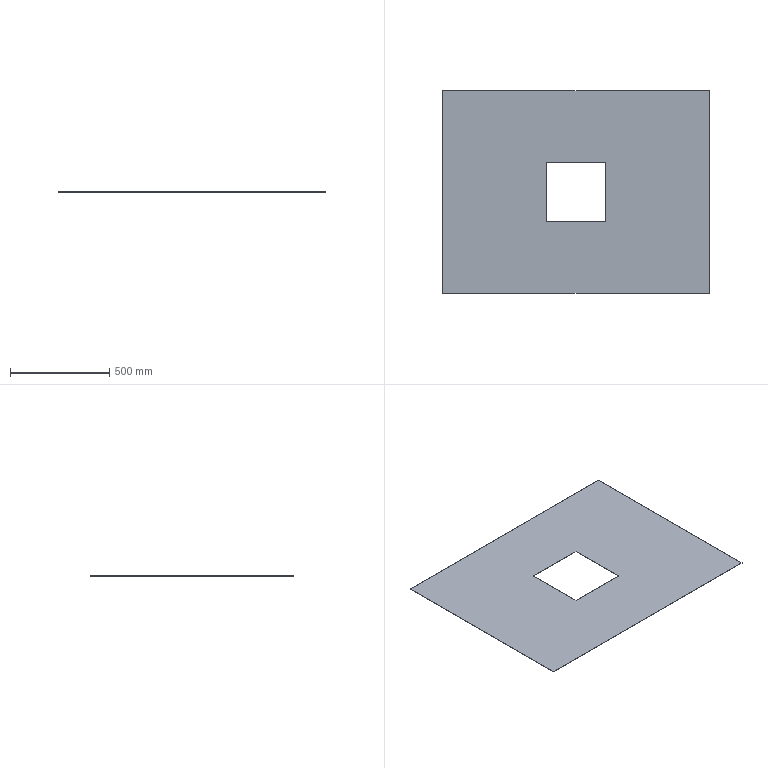Part | SolidWorks | features FlatPattern 1, SMBaseFlange 1, SheetMetal 1 | 1 solid | 10 faces | box 1345 x 1022 x 1.5 mm | volume 1927692 mm3 | plane 10
STEP:
#1=CARTESIAN_POINT('',(-672.5,0.,1.5));
#2=VERTEX_POINT('',#1);
#3=CARTESIAN_POINT('',(-672.5,-1022.4,1.5));
#4=VERTEX_POINT('',#3);
#5=CARTESIAN_POINT('',(-672.5,0.,1.5));
#6=DIRECTION('',(0.,-1.,0.));
#7=VECTOR('',#6,1000.);
#8=LINE('',#5,#7);
#9=EDGE_CURVE('',#2,#4,#8,.T.);
#10=ORIENTED_EDGE('',*,*,#9,.T.);
#11=CARTESIAN_POINT('',(672.5,-1022.4,1.5));
#12=VERTEX_POINT('',#11);
#13=CARTESIAN_POINT('',(-672.5,-1022.4,1.5));
#14=DIRECTION('',(1.,0.,0.));
#15=VECTOR('',#14,1000.);
#16=LINE('',#13,#15);
#17=EDGE_CURVE('',#4,#12,#16,.T.);
#18=ORIENTED_EDGE('',*,*,#17,.T.);
#19=CARTESIAN_POINT('',(672.5,0.,1.5));
#20=VERTEX_POINT('',#19);
#21=CARTESIAN_POINT('',(672.5,0.,1.5));
#22=DIRECTION('',(0.,1.,0.));
#23=VECTOR('',#22,1000.);
#24=LINE('',#21,#23);
#25=EDGE_CURVE('',#12,#20,#24,.T.);
#26=ORIENTED_EDGE('',*,*,#25,.T.);
#27=CARTESIAN_POINT('',(-672.5,0.,1.5));
#28=DIRECTION('',(-1.,0.,0.));
#29=VECTOR('',#28,1000.);
#30=LINE('',#27,#29);
#31=EDGE_CURVE('',#20,#2,#30,.T.);
#32=ORIENTED_EDGE('',*,*,#31,.T.);
#33=EDGE_LOOP('',(#10,#18,#26,#32));
#34=FACE_OUTER_BOUND('',#33,.T.);
#35=CARTESIAN_POINT('',(150.,-361.2,1.5));
#36=VERTEX_POINT('',#35);
#37=CARTESIAN_POINT('',(-150.,-361.2,1.5));
#38=VERTEX_POINT('',#37);
#39=CARTESIAN_POINT('',(-150.,-361.2,1.5));
#40=DIRECTION('',(-1.,0.,0.));
#41=VECTOR('',#40,1000.);
#42=LINE('',#39,#41);
#43=EDGE_CURVE('',#36,#38,#42,.T.);
#44=ORIENTED_EDGE('',*,*,#43,.F.);
#45=CARTESIAN_POINT('',(150.,-661.2,1.5));
#46=VERTEX_POINT('',#45);
#47=CARTESIAN_POINT('',(150.,-661.2,1.5));
#48=DIRECTION('',(0.,1.,0.));
#49=VECTOR('',#48,1000.);
#50=LINE('',#47,#49);
#51=EDGE_CURVE('',#46,#36,#50,.T.);
#52=ORIENTED_EDGE('',*,*,#51,.F.);
#53=CARTESIAN_POINT('',(-150.,-661.2,1.5));
#54=VERTEX_POINT('',#53);
#55=CARTESIAN_POINT('',(-150.,-661.2,1.5));
#56=DIRECTION('',(1.,0.,0.));
#57=VECTOR('',#56,1000.);
#58=LINE('',#55,#57);
#59=EDGE_CURVE('',#54,#46,#58,.T.);
#60=ORIENTED_EDGE('',*,*,#59,.F.);
#61=CARTESIAN_POINT('',(-150.,-661.2,1.5));
#62=DIRECTION('',(0.,-1.,0.));
#63=VECTOR('',#62,1000.);
#64=LINE('',#61,#63);
#65=EDGE_CURVE('',#38,#54,#64,.T.);
#66=ORIENTED_EDGE('',*,*,#65,.F.);
#67=EDGE_LOOP('',(#44,#52,#60,#66));
#68=FACE_BOUND('',#67,.T.);
#69=CARTESIAN_POINT('',(0.,0.,1.5));
#70=DIRECTION('',(0.,0.,1.));
#71=DIRECTION('',(1.,0.,0.));
#72=AXIS2_PLACEMENT_3D('',#69,#70,#71);
#73=PLANE('',#72);
#74=ADVANCED_FACE('',(#34,#68),#73,.T.);
#75=CARTESIAN_POINT('',(-672.5,0.,0.));
#76=VERTEX_POINT('',#75);
#77=CARTESIAN_POINT('',(-672.5,-1022.4,0.));
#78=VERTEX_POINT('',#77);
#79=CARTESIAN_POINT('',(-672.5,0.,0.));
#80=DIRECTION('',(0.,-1.,0.));
#81=VECTOR('',#80,1000.);
#82=LINE('',#79,#81);
#83=EDGE_CURVE('',#76,#78,#82,.T.);
#84=ORIENTED_EDGE('',*,*,#83,.F.);
#85=CARTESIAN_POINT('',(672.5,0.,0.));
#86=VERTEX_POINT('',#85);
#87=CARTESIAN_POINT('',(-672.5,0.,0.));
#88=DIRECTION('',(-1.,0.,0.));
#89=VECTOR('',#88,1000.);
#90=LINE('',#87,#89);
#91=EDGE_CURVE('',#86,#76,#90,.T.);
#92=ORIENTED_EDGE('',*,*,#91,.F.);
#93=CARTESIAN_POINT('',(672.5,-1022.4,0.));
#94=VERTEX_POINT('',#93);
#95=CARTESIAN_POINT('',(672.5,0.,0.));
#96=DIRECTION('',(0.,1.,0.));
#97=VECTOR('',#96,1000.);
#98=LINE('',#95,#97);
#99=EDGE_CURVE('',#94,#86,#98,.T.);
#100=ORIENTED_EDGE('',*,*,#99,.F.);
#101=CARTESIAN_POINT('',(-672.5,-1022.4,0.));
#102=DIRECTION('',(1.,0.,0.));
#103=VECTOR('',#102,1000.);
#104=LINE('',#101,#103);
#105=EDGE_CURVE('',#78,#94,#104,.T.);
#106=ORIENTED_EDGE('',*,*,#105,.F.);
#107=EDGE_LOOP('',(#84,#92,#100,#106));
#108=FACE_OUTER_BOUND('',#107,.T.);
#109=CARTESIAN_POINT('',(150.,-661.2,0.));
#110=VERTEX_POINT('',#109);
#111=CARTESIAN_POINT('',(150.,-361.2,0.));
#112=VERTEX_POINT('',#111);
#113=CARTESIAN_POINT('',(150.,-661.2,0.));
#114=DIRECTION('',(0.,1.,0.));
#115=VECTOR('',#114,1000.);
#116=LINE('',#113,#115);
#117=EDGE_CURVE('',#110,#112,#116,.T.);
#118=ORIENTED_EDGE('',*,*,#117,.T.);
#119=CARTESIAN_POINT('',(-150.,-361.2,0.));
#120=VERTEX_POINT('',#119);
#121=CARTESIAN_POINT('',(-150.,-361.2,0.));
#122=DIRECTION('',(-1.,0.,0.));
#123=VECTOR('',#122,1000.);
#124=LINE('',#121,#123);
#125=EDGE_CURVE('',#112,#120,#124,.T.);
#126=ORIENTED_EDGE('',*,*,#125,.T.);
#127=CARTESIAN_POINT('',(-150.,-661.2,0.));
#128=VERTEX_POINT('',#127);
#129=CARTESIAN_POINT('',(-150.,-661.2,0.));
#130=DIRECTION('',(0.,-1.,0.));
#131=VECTOR('',#130,1000.);
#132=LINE('',#129,#131);
#133=EDGE_CURVE('',#120,#128,#132,.T.);
#134=ORIENTED_EDGE('',*,*,#133,.T.);
#135=CARTESIAN_POINT('',(-150.,-661.2,0.));
#136=DIRECTION('',(1.,0.,0.));
#137=VECTOR('',#136,1000.);
#138=LINE('',#135,#137);
#139=EDGE_CURVE('',#128,#110,#138,.T.);
#140=ORIENTED_EDGE('',*,*,#139,.T.);
#141=EDGE_LOOP('',(#118,#126,#134,#140));
#142=FACE_BOUND('',#141,.T.);
#143=CARTESIAN_POINT('',(0.,0.,0.));
#144=DIRECTION('',(0.,0.,1.));
#145=DIRECTION('',(1.,0.,0.));
#146=AXIS2_PLACEMENT_3D('',#143,#144,#145);
#147=PLANE('',#146);
#148=ADVANCED_FACE('',(#108,#142),#147,.F.);
#149=ORIENTED_EDGE('',*,*,#83,.T.);
#150=CARTESIAN_POINT('',(-672.5,-1022.4,1.5));
#151=DIRECTION('',(0.,0.,-1.));
#152=VECTOR('',#151,1000.);
#153=LINE('',#150,#152);
#154=EDGE_CURVE('',#4,#78,#153,.T.);
#155=ORIENTED_EDGE('',*,*,#154,.F.);
#156=ORIENTED_EDGE('',*,*,#9,.F.);
#157=CARTESIAN_POINT('',(-672.5,0.,1.5));
#158=DIRECTION('',(0.,0.,-1.));
#159=VECTOR('',#158,1000.);
#160=LINE('',#157,#159);
#161=EDGE_CURVE('',#2,#76,#160,.T.);
#162=ORIENTED_EDGE('',*,*,#161,.T.);
#163=EDGE_LOOP('',(#149,#155,#156,#162));
#164=FACE_OUTER_BOUND('',#163,.T.);
#165=CARTESIAN_POINT('',(-672.5,0.,1.5));
#166=DIRECTION('',(1.,0.,0.));
#167=DIRECTION('',(0.,0.,-1.));
#168=AXIS2_PLACEMENT_3D('',#165,#166,#167);
#169=PLANE('',#168);
#170=ADVANCED_FACE('',(#164),#169,.F.);
#171=ORIENTED_EDGE('',*,*,#105,.T.);
#172=CARTESIAN_POINT('',(672.5,-1022.4,1.5));
#173=DIRECTION('',(0.,0.,-1.));
#174=VECTOR('',#173,1000.);
#175=LINE('',#172,#174);
#176=EDGE_CURVE('',#12,#94,#175,.T.);
#177=ORIENTED_EDGE('',*,*,#176,.F.);
#178=ORIENTED_EDGE('',*,*,#17,.F.);
#179=ORIENTED_EDGE('',*,*,#154,.T.);
#180=EDGE_LOOP('',(#171,#177,#178,#179));
#181=FACE_OUTER_BOUND('',#180,.T.);
#182=CARTESIAN_POINT('',(-672.5,-1022.4,1.5));
#183=DIRECTION('',(0.,1.,0.));
#184=DIRECTION('',(0.,0.,1.));
#185=AXIS2_PLACEMENT_3D('',#182,#183,#184);
#186=PLANE('',#185);
#187=ADVANCED_FACE('',(#181),#186,.F.);
#188=ORIENTED_EDGE('',*,*,#99,.T.);
#189=CARTESIAN_POINT('',(672.5,0.,1.5));
#190=DIRECTION('',(0.,0.,-1.));
#191=VECTOR('',#190,1000.);
#192=LINE('',#189,#191);
#193=EDGE_CURVE('',#20,#86,#192,.T.);
#194=ORIENTED_EDGE('',*,*,#193,.F.);
#195=ORIENTED_EDGE('',*,*,#25,.F.);
#196=ORIENTED_EDGE('',*,*,#176,.T.);
#197=EDGE_LOOP('',(#188,#194,#195,#196));
#198=FACE_OUTER_BOUND('',#197,.T.);
#199=CARTESIAN_POINT('',(672.5,0.,1.5));
#200=DIRECTION('',(-1.,0.,0.));
#201=DIRECTION('',(0.,0.,1.));
#202=AXIS2_PLACEMENT_3D('',#199,#200,#201);
#203=PLANE('',#202);
#204=ADVANCED_FACE('',(#198),#203,.F.);
#205=ORIENTED_EDGE('',*,*,#91,.T.);
#206=ORIENTED_EDGE('',*,*,#161,.F.);
#207=ORIENTED_EDGE('',*,*,#31,.F.);
#208=ORIENTED_EDGE('',*,*,#193,.T.);
#209=EDGE_LOOP('',(#205,#206,#207,#208));
#210=FACE_OUTER_BOUND('',#209,.T.);
#211=CARTESIAN_POINT('',(-672.5,0.,1.5));
#212=DIRECTION('',(0.,-1.,0.));
#213=DIRECTION('',(0.,0.,-1.));
#214=AXIS2_PLACEMENT_3D('',#211,#212,#213);
#215=PLANE('',#214);
#216=ADVANCED_FACE('',(#210),#215,.F.);
#217=ORIENTED_EDGE('',*,*,#117,.F.);
#218=CARTESIAN_POINT('',(150.,-661.2,1.5));
#219=DIRECTION('',(0.,0.,-1.));
#220=VECTOR('',#219,1000.);
#221=LINE('',#218,#220);
#222=EDGE_CURVE('',#46,#110,#221,.T.);
#223=ORIENTED_EDGE('',*,*,#222,.F.);
#224=ORIENTED_EDGE('',*,*,#51,.T.);
#225=CARTESIAN_POINT('',(150.,-361.2,1.5));
#226=DIRECTION('',(0.,0.,-1.));
#227=VECTOR('',#226,1000.);
#228=LINE('',#225,#227);
#229=EDGE_CURVE('',#36,#112,#228,.T.);
#230=ORIENTED_EDGE('',*,*,#229,.T.);
#231=EDGE_LOOP('',(#217,#223,#224,#230));
#232=FACE_OUTER_BOUND('',#231,.T.);
#233=CARTESIAN_POINT('',(150.,-661.2,1.5));
#234=DIRECTION('',(-1.,0.,0.));
#235=DIRECTION('',(0.,-1.,0.));
#236=AXIS2_PLACEMENT_3D('',#233,#234,#235);
#237=PLANE('',#236);
#238=ADVANCED_FACE('',(#232),#237,.T.);
#239=ORIENTED_EDGE('',*,*,#125,.F.);
#240=ORIENTED_EDGE('',*,*,#229,.F.);
#241=ORIENTED_EDGE('',*,*,#43,.T.);
#242=CARTESIAN_POINT('',(-150.,-361.2,1.5));
#243=DIRECTION('',(0.,0.,-1.));
#244=VECTOR('',#243,1000.);
#245=LINE('',#242,#244);
#246=EDGE_CURVE('',#38,#120,#245,.T.);
#247=ORIENTED_EDGE('',*,*,#246,.T.);
#248=EDGE_LOOP('',(#239,#240,#241,#247));
#249=FACE_OUTER_BOUND('',#248,.T.);
#250=CARTESIAN_POINT('',(-150.,-361.2,1.5));
#251=DIRECTION('',(0.,-1.,0.));
#252=DIRECTION('',(1.,0.,0.));
#253=AXIS2_PLACEMENT_3D('',#250,#251,#252);
#254=PLANE('',#253);
#255=ADVANCED_FACE('',(#249),#254,.T.);
#256=ORIENTED_EDGE('',*,*,#133,.F.);
#257=ORIENTED_EDGE('',*,*,#246,.F.);
#258=ORIENTED_EDGE('',*,*,#65,.T.);
#259=CARTESIAN_POINT('',(-150.,-661.2,1.5));
#260=DIRECTION('',(0.,0.,-1.));
#261=VECTOR('',#260,1000.);
#262=LINE('',#259,#261);
#263=EDGE_CURVE('',#54,#128,#262,.T.);
#264=ORIENTED_EDGE('',*,*,#263,.T.);
#265=EDGE_LOOP('',(#256,#257,#258,#264));
#266=FACE_OUTER_BOUND('',#265,.T.);
#267=CARTESIAN_POINT('',(-150.,-661.2,1.5));
#268=DIRECTION('',(1.,0.,0.));
#269=DIRECTION('',(0.,0.,-1.));
#270=AXIS2_PLACEMENT_3D('',#267,#268,#269);
#271=PLANE('',#270);
#272=ADVANCED_FACE('',(#266),#271,.T.);
#273=ORIENTED_EDGE('',*,*,#139,.F.);
#274=ORIENTED_EDGE('',*,*,#263,.F.);
#275=ORIENTED_EDGE('',*,*,#59,.T.);
#276=ORIENTED_EDGE('',*,*,#222,.T.);
#277=EDGE_LOOP('',(#273,#274,#275,#276));
#278=FACE_OUTER_BOUND('',#277,.T.);
#279=CARTESIAN_POINT('',(-150.,-661.2,1.5));
#280=DIRECTION('',(0.,1.,0.));
#281=DIRECTION('',(0.,0.,1.));
#282=AXIS2_PLACEMENT_3D('',#279,#280,#281);
#283=PLANE('',#282);
#284=ADVANCED_FACE('',(#278),#283,.T.);
#285=CLOSED_SHELL('',(#74,#148,#170,#187,#204,#216,#238,#255,#272,#284));
#286=MANIFOLD_SOLID_BREP('',#285);
#287=CARTESIAN_POINT('',(0.,0.,0.));
#288=DIRECTION('',(0.,0.,1.));
#289=DIRECTION('',(1.,0.,0.));
#290=AXIS2_PLACEMENT_3D('',#287,#288,#289);
#291=(LENGTH_UNIT()NAMED_UNIT(*)SI_UNIT(.MILLI.,.METRE.));
#292=UNCERTAINTY_MEASURE_WITH_UNIT(LENGTH_MEASURE(0.00001),#291,'','');
#293=(NAMED_UNIT(*)PLANE_ANGLE_UNIT()SI_UNIT($,.RADIAN.));
#294=(NAMED_UNIT(*)SI_UNIT($,.STERADIAN.)SOLID_ANGLE_UNIT());
#295=(GEOMETRIC_REPRESENTATION_CONTEXT(3)GLOBAL_UNCERTAINTY_ASSIGNED_CONTEXT((#292))GLOBAL_UNIT_ASSIGNED_CONTEXT((#291,#293,#294))REPRESENTATION_CONTEXT('',''));
#296=ADVANCED_BREP_SHAPE_REPRESENTATION('',(#286,#290),#295);